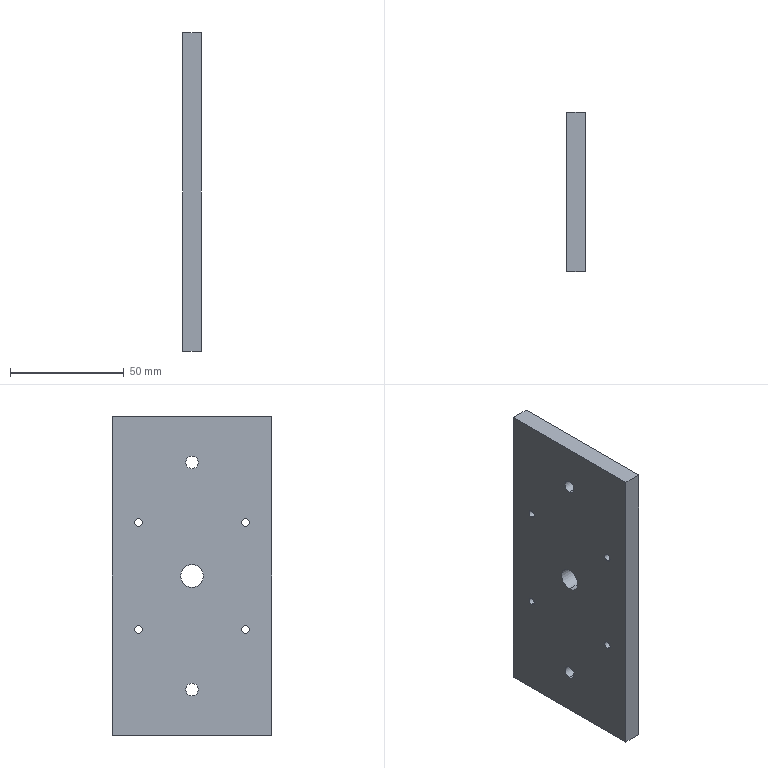Part | STEP file | 03-05 Motor fixing plate | 1 solid | 20 faces | box 8 x 70 x 140 mm | volume 77118 mm3 | cylinder 14 | plane 6 | commonest cylinder face diameters 3.3 x8 5.5 x4 10 x2